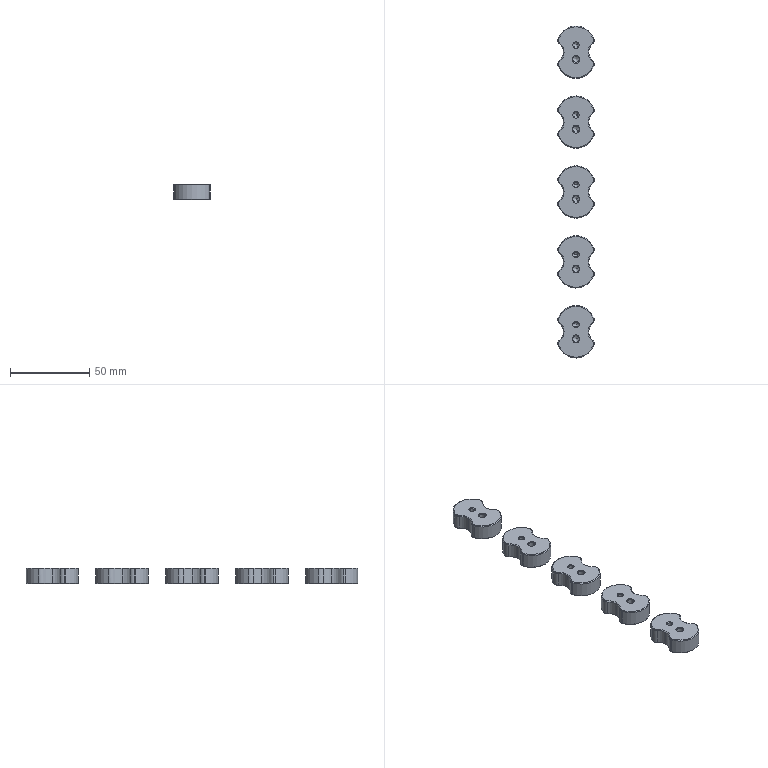NC program | NX | posted with a generic post | part box 22.923 x 209 x 10 mm
Lines 19 to 811 of 9354:
(ZLEVEL_PROFILE_COPY_1 , TOOL : D10)
N36 T15 M6
N38 G54
N40 G17 G0 G90 X-101.822 Y14.358 S9500 M3
N42 G43 Z30. H15
N44 Z1.5
N46 G94 G1 X-101.702 Y14.449 Z1.492 F1000.
N48 X-99.279 Y15.732 Z1.348
N50 X-97.67 Y16.315 Z1.259
N52 X-96.247 Y16.563 Z1.183
N54 X-94.852 Y16.56 Z1.11
N56 X-93.039 Y16.189 Z1.013
N58 X-91.358 Y15.417 Z0.916
N60 X-89.894 Y14.286 Z0.819
N62 X-89.216 Y13.501 Z0.765
N64 X-88.351 Y13.102 Z0.715
N66 X-87.673 Y13.098 Z0.679
N68 X-87.202 Y13.242 Z0.653
N70 X-86.784 Y13.501 Z0.628
N72 X-86.106 Y14.286 Z0.573
N74 X-84.79 Y15.326 Z0.485
N76 X-83.287 Y16.074 Z0.397
N78 X-81.663 Y16.498 Z0.309
N80 X-79.987 Y16.579 Z0.221
N82 X-78.33 Y16.315 Z0.134
N84 X-76.721 Y15.732 Z0.044
N86 X-74.333 Y14.471 Z-0.098
N88 X-72.173 Y12.85 Z-0.239
N90 X-70.294 Y10.91 Z-0.381
N92 X-68.743 Y8.699 Z-0.522
N94 X-67.559 Y6.272 Z-0.664
N96 X-66.772 Y3.688 Z-0.805
N98 X-66.4 Y1.013 Z-0.947
N100 Y0. Z-1.
N102 G2 X-77.674 Y-16.077 R17.1 F3500.
N104 X-86.562 Y-13.758 R8.1
N106 G3 X-89.438 Y-13.758 R1.9
N108 G2 X-98.326 Y-16.077 R8.1
N110 X-98.326 Y16.077 R17.1
N112 X-89.438 Y13.758 R8.1
N114 G3 X-86.562 Y13.758 R1.9
N116 G2 X-77.674 Y16.077 R8.1
N118 X-66.4 Y0. R17.1
N120 G1 X-66.422 Y-0.858 Z-1.007
N122 X-66.486 Y-1.714 Z-1.013
N124 X-66.609 Y-2.666 Z-1.021
N126 X-66.785 Y-3.61 Z-1.028
N128 X-67.014 Y-4.542 Z-1.036
N130 X-67.295 Y-5.46 Z-1.043
N132 X-67.627 Y-6.36 Z-1.05
N134 X-68.009 Y-7.241 Z-1.058
N136 X-68.439 Y-8.098 Z-1.065
N138 X-68.917 Y-8.931 Z-1.073
N140 X-69.441 Y-9.735 Z-1.08
N142 X-70.01 Y-10.508 Z-1.088
N144 X-70.621 Y-11.249 Z-1.095
N146 X-71.272 Y-11.954 Z-1.102
N148 X-71.962 Y-12.621 Z-1.11
N150 X-72.688 Y-13.248 Z-1.117
N152 X-73.449 Y-13.834 Z-1.125
N154 X-74.241 Y-14.376 Z-1.132
N156 X-75.062 Y-14.873 Z-1.14
N158 X-75.91 Y-15.323 Z-1.147
N160 X-76.781 Y-15.725 Z-1.154
N162 X-77.674 Y-16.077 Z-1.162
N164 X-78.255 Y-16.263 Z-1.167
N166 X-78.849 Y-16.405 Z-1.171
N168 X-79.451 Y-16.502 Z-1.176
N170 X-80.06 Y-16.553 Z-1.181
N172 X-80.67 Y-16.558 Z-1.185
N174 X-81.279 Y-16.517 Z-1.19
N176 X-81.883 Y-16.431 Z-1.195
N178 X-82.479 Y-16.299 Z-1.2
N180 X-83.063 Y-16.123 Z-1.204
N182 X-83.632 Y-15.903 Z-1.209
N184 X-84.184 Y-15.641 Z-1.214
N186 X-84.714 Y-15.339 Z-1.219
N188 X-85.219 Y-14.997 Z-1.223
N190 X-85.698 Y-14.618 Z-1.228
N192 X-86.146 Y-14.204 Z-1.233
N194 X-86.562 Y-13.758 Z-1.237
N196 X-86.909 Y-13.444 Z-1.241
N198 X-87.064 Y-13.346 Z-1.242
N200 X-87.429 Y-13.188 Z-1.246
N202 X-87.676 Y-13.128 Z-1.247
N204 X-88.058 Y-13.101 Z-1.25
N206 X-88.324 Y-13.128 Z-1.253
N208 X-88.692 Y-13.23 Z-1.255
N210 X-88.936 Y-13.346 Z-1.258
N212 X-89.08 Y-13.437 Z-1.259
N214 X-89.438 Y-13.758 Z-1.263
N216 X-89.913 Y-14.262 Z-1.268
N218 X-90.43 Y-14.724 Z-1.273
N220 X-90.984 Y-15.141 Z-1.279
N222 X-91.572 Y-15.508 Z-1.284
N224 X-92.189 Y-15.824 Z-1.289
N226 X-92.831 Y-16.086 Z-1.295
N228 X-93.493 Y-16.292 Z-1.3
N230 X-94.17 Y-16.44 Z-1.305
N232 X-94.857 Y-16.53 Z-1.311
N234 X-95.55 Y-16.562 Z-1.316
N236 X-96.021 Y-16.549 Z-1.32
N238 X-96.492 Y-16.509 Z-1.323
N240 X-96.959 Y-16.441 Z-1.327
N242 X-97.421 Y-16.346 Z-1.331
N244 X-97.878 Y-16.225 Z-1.334
N246 X-98.326 Y-16.077 Z-1.338
N248 X-98.977 Y-15.826 Z-1.344
N250 X-99.617 Y-15.549 Z-1.349
N252 X-100.245 Y-15.245 Z-1.354
N254 X-100.861 Y-14.917 Z-1.36
N256 X-101.462 Y-14.563 Z-1.365
N258 X-102.048 Y-14.186 Z-1.371
N260 X-102.854 Y-13.609 Z-1.378
N262 X-103.624 Y-12.987 Z-1.386
N264 X-104.358 Y-12.321 Z-1.394
N266 X-105.051 Y-11.614 Z-1.401
N268 X-105.703 Y-10.867 Z-1.409
N270 X-106.31 Y-10.085 Z-1.417
N272 X-106.87 Y-9.268 Z-1.424
N274 X-107.383 Y-8.421 Z-1.432
N276 X-107.846 Y-7.545 Z-1.44
N278 X-108.257 Y-6.643 Z-1.447
N280 X-108.615 Y-5.72 Z-1.455
N282 X-108.919 Y-4.777 Z-1.463
N284 X-109.168 Y-3.819 Z-1.47
N286 X-109.361 Y-2.847 Z-1.478
N288 X-109.498 Y-1.866 Z-1.486
N290 X-109.577 Y-0.879 Z-1.493
N292 X-109.6 Y0.112 Z-1.501
N294 X-109.564 Y1.101 Z-1.509
N296 X-109.472 Y2.088 Z-1.516
N298 X-109.323 Y3.067 Z-1.524
N300 X-109.117 Y4.036 Z-1.532
N302 X-108.855 Y4.991 Z-1.539
N304 X-108.539 Y5.93 Z-1.547
N306 X-108.169 Y6.849 Z-1.555
N308 X-107.746 Y7.744 Z-1.562
N310 X-107.272 Y8.614 Z-1.57
N312 X-106.748 Y9.455 Z-1.578
N314 X-106.177 Y10.264 Z-1.585
N316 X-105.56 Y11.039 Z-1.593
N318 X-104.899 Y11.776 Z-1.601
N320 X-104.196 Y12.475 Z-1.608
N322 X-103.454 Y13.131 Z-1.616
N324 X-102.675 Y13.743 Z-1.624
N326 X-101.863 Y14.309 Z-1.631
N328 X-101.018 Y14.827 Z-1.639
N330 X-100.146 Y15.296 Z-1.647
N332 X-99.247 Y15.713 Z-1.654
N334 X-98.326 Y16.077 Z-1.662
N336 X-97.878 Y16.225 Z-1.666
N338 X-97.421 Y16.346 Z-1.669
N340 X-96.959 Y16.441 Z-1.673
N342 X-96.492 Y16.509 Z-1.676
N344 X-96.021 Y16.549 Z-1.68
N346 X-95.55 Y16.562 Z-1.684
N348 X-94.857 Y16.53 Z-1.689
N350 X-94.17 Y16.44 Z-1.695
N352 X-93.493 Y16.292 Z-1.7
N354 X-92.831 Y16.086 Z-1.705
N356 X-92.189 Y15.824 Z-1.711
N358 X-91.572 Y15.508 Z-1.716
N360 X-90.984 Y15.141 Z-1.721
N362 X-90.43 Y14.724 Z-1.727
N364 X-89.913 Y14.262 Z-1.732
N366 X-89.438 Y13.758 Z-1.737
N368 X-89.146 Y13.485 Z-1.74
N370 X-89.032 Y13.405 Z-1.742
N372 X-88.74 Y13.25 Z-1.744
N374 X-88.544 Y13.179 Z-1.746
N376 X-88.23 Y13.114 Z-1.748
N378 X-88.012 Y13.1 Z-1.75
N380 X-87.691 Y13.125 Z-1.752
N382 X-87.471 Y13.175 Z-1.754
N384 X-87.172 Y13.29 Z-1.757
N386 X-86.975 Y13.4 Z-1.758
N388 X-86.756 Y13.564 Z-1.76
N390 X-86.562 Y13.758 Z-1.763
N392 X-86.146 Y14.204 Z-1.767
N394 X-85.698 Y14.618 Z-1.772
N396 X-85.219 Y14.997 Z-1.777
N398 X-84.714 Y15.339 Z-1.781
N400 X-84.184 Y15.641 Z-1.786
N402 X-83.632 Y15.903 Z-1.791
N404 X-83.063 Y16.123 Z-1.796
N406 X-82.479 Y16.299 Z-1.8
N408 X-81.883 Y16.431 Z-1.805
N410 X-81.279 Y16.517 Z-1.81
N412 X-80.67 Y16.558 Z-1.815
N414 X-80.06 Y16.553 Z-1.819
N416 X-79.451 Y16.502 Z-1.824
N418 X-78.849 Y16.405 Z-1.829
N420 X-78.255 Y16.263 Z-1.833
N422 X-77.674 Y16.077 Z-1.838
N424 X-76.79 Y15.728 Z-1.845
N426 X-75.926 Y15.331 Z-1.853
N428 X-75.086 Y14.887 Z-1.86
N430 X-74.272 Y14.396 Z-1.868
N432 X-73.486 Y13.861 Z-1.875
N434 X-72.731 Y13.283 Z-1.882
N436 X-72.01 Y12.664 Z-1.89
N438 X-71.324 Y12.006 Z-1.897
N440 X-70.675 Y11.311 Z-1.904
N442 X-70.067 Y10.581 Z-1.912
N444 X-69.499 Y9.818 Z-1.919
N446 X-68.975 Y9.025 Z-1.926
N448 X-68.496 Y8.204 Z-1.934
N450 X-68.064 Y7.357 Z-1.941
N452 X-67.679 Y6.488 Z-1.948
N454 X-67.343 Y5.599 Z-1.956
N456 X-67.056 Y4.693 Z-1.963
N458 X-66.821 Y3.772 Z-1.971
N460 X-66.637 Y2.839 Z-1.978
N462 X-66.506 Y1.898 Z-1.985
N464 X-66.426 Y0.95 Z-1.993
N466 X-66.4 Y0. Z-2.
N468 X-66.422 Y-0.858 Z-2.007
N470 X-66.486 Y-1.714 Z-2.013
N472 X-66.609 Y-2.666 Z-2.021
N474 X-66.785 Y-3.61 Z-2.028
N476 X-67.014 Y-4.542 Z-2.036
N478 X-67.295 Y-5.46 Z-2.043
N480 X-67.627 Y-6.36 Z-2.05
N482 X-68.009 Y-7.241 Z-2.058
N484 X-68.439 Y-8.098 Z-2.065
N486 X-68.917 Y-8.931 Z-2.073
N488 X-69.441 Y-9.735 Z-2.08
N490 X-70.01 Y-10.508 Z-2.088
N492 X-70.621 Y-11.249 Z-2.095
N494 X-71.272 Y-11.954 Z-2.102
N496 X-71.962 Y-12.621 Z-2.11
N498 X-72.688 Y-13.248 Z-2.117
N500 X-73.449 Y-13.834 Z-2.125
N502 X-74.241 Y-14.376 Z-2.132
N504 X-75.062 Y-14.873 Z-2.14
N506 X-75.91 Y-15.323 Z-2.147
N508 X-76.781 Y-15.725 Z-2.154
N510 X-77.674 Y-16.077 Z-2.162
N512 X-78.255 Y-16.263 Z-2.167
N514 X-78.849 Y-16.405 Z-2.171
N516 X-79.451 Y-16.502 Z-2.176
N518 X-80.06 Y-16.553 Z-2.181
N520 X-80.67 Y-16.558 Z-2.185
N522 X-81.279 Y-16.517 Z-2.19
N524 X-81.883 Y-16.431 Z-2.195
N526 X-82.479 Y-16.299 Z-2.2
N528 X-83.063 Y-16.123 Z-2.204
N530 X-83.632 Y-15.903 Z-2.209
N532 X-84.184 Y-15.641 Z-2.214
N534 X-84.714 Y-15.339 Z-2.219
N536 X-85.219 Y-14.997 Z-2.223
N538 X-85.698 Y-14.618 Z-2.228
N540 X-86.146 Y-14.204 Z-2.233
N542 X-86.562 Y-13.758 Z-2.237
N544 X-86.909 Y-13.444 Z-2.241
N546 X-87.064 Y-13.346 Z-2.242
N548 X-87.429 Y-13.188 Z-2.246
N550 X-87.676 Y-13.128 Z-2.247
N552 X-88.058 Y-13.101 Z-2.25
N554 X-88.324 Y-13.128 Z-2.253
N556 X-88.692 Y-13.23 Z-2.255
N558 X-88.936 Y-13.346 Z-2.258
N560 X-89.08 Y-13.437 Z-2.259
N562 X-89.438 Y-13.758 Z-2.263
N564 X-89.913 Y-14.262 Z-2.268
N566 X-90.43 Y-14.724 Z-2.273
N568 X-90.984 Y-15.141 Z-2.279
N570 X-91.572 Y-15.508 Z-2.284
N572 X-92.189 Y-15.824 Z-2.289
N574 X-92.831 Y-16.086 Z-2.295
N576 X-93.493 Y-16.292 Z-2.3
N578 X-94.17 Y-16.44 Z-2.305
N580 X-94.857 Y-16.53 Z-2.311
N582 X-95.55 Y-16.562 Z-2.316
N584 X-96.021 Y-16.549 Z-2.32
N586 X-96.492 Y-16.509 Z-2.323
N588 X-96.959 Y-16.441 Z-2.327
N590 X-97.421 Y-16.346 Z-2.331
N592 X-97.878 Y-16.225 Z-2.334
N594 X-98.326 Y-16.077 Z-2.338
N596 X-98.977 Y-15.826 Z-2.344
N598 X-99.617 Y-15.549 Z-2.349
N600 X-100.245 Y-15.245 Z-2.354
N602 X-100.861 Y-14.917 Z-2.36
N604 X-101.462 Y-14.563 Z-2.365
N606 X-102.048 Y-14.186 Z-2.371
N608 X-102.854 Y-13.609 Z-2.378
N610 X-103.624 Y-12.987 Z-2.386
N612 X-104.358 Y-12.321 Z-2.394
N614 X-105.051 Y-11.614 Z-2.401
N616 X-105.703 Y-10.867 Z-2.409
N618 X-106.31 Y-10.085 Z-2.417
N620 X-106.87 Y-9.268 Z-2.424
N622 X-107.383 Y-8.421 Z-2.432
N624 X-107.846 Y-7.545 Z-2.44
N626 X-108.257 Y-6.643 Z-2.447
N628 X-108.615 Y-5.72 Z-2.455
N630 X-108.919 Y-4.777 Z-2.463
N632 X-109.168 Y-3.819 Z-2.47
N634 X-109.361 Y-2.847 Z-2.478
N636 X-109.498 Y-1.866 Z-2.486
N638 X-109.577 Y-0.879 Z-2.493
N640 X-109.6 Y0.112 Z-2.501
N642 X-109.564 Y1.101 Z-2.509
N644 X-109.472 Y2.088 Z-2.516
N646 X-109.323 Y3.067 Z-2.524
N648 X-109.117 Y4.036 Z-2.532
N650 X-108.855 Y4.991 Z-2.539
N652 X-108.539 Y5.93 Z-2.547
N654 X-108.169 Y6.849 Z-2.555
N656 X-107.746 Y7.744 Z-2.562
N658 X-107.272 Y8.614 Z-2.57
N660 X-106.748 Y9.455 Z-2.578
N662 X-106.177 Y10.264 Z-2.585
N664 X-105.56 Y11.039 Z-2.593
N666 X-104.899 Y11.776 Z-2.601
N668 X-104.196 Y12.475 Z-2.608
N670 X-103.454 Y13.131 Z-2.616
N672 X-102.675 Y13.743 Z-2.624
N674 X-101.863 Y14.309 Z-2.631
N676 X-101.018 Y14.827 Z-2.639
N678 X-100.146 Y15.296 Z-2.647
N680 X-99.247 Y15.713 Z-2.654
N682 X-98.326 Y16.077 Z-2.662
N684 X-97.878 Y16.225 Z-2.666
N686 X-97.421 Y16.346 Z-2.669
N688 X-96.959 Y16.441 Z-2.673
N690 X-96.492 Y16.509 Z-2.676
N692 X-96.021 Y16.549 Z-2.68
N694 X-95.55 Y16.562 Z-2.684
N696 X-94.857 Y16.53 Z-2.689
N698 X-94.17 Y16.44 Z-2.695
N700 X-93.493 Y16.292 Z-2.7
N702 X-92.831 Y16.086 Z-2.705
N704 X-92.189 Y15.824 Z-2.711
N706 X-91.572 Y15.508 Z-2.716
N708 X-90.984 Y15.141 Z-2.721
N710 X-90.43 Y14.724 Z-2.727
N712 X-89.913 Y14.262 Z-2.732
N714 X-89.438 Y13.758 Z-2.737
N716 X-89.146 Y13.485 Z-2.74
N718 X-89.032 Y13.405 Z-2.742
N720 X-88.74 Y13.25 Z-2.744
N722 X-88.544 Y13.179 Z-2.746
N724 X-88.23 Y13.114 Z-2.748
N726 X-88.012 Y13.1 Z-2.75
N728 X-87.691 Y13.125 Z-2.752
N730 X-87.471 Y13.175 Z-2.754
N732 X-87.172 Y13.29 Z-2.757
N734 X-86.975 Y13.4 Z-2.758
N736 X-86.756 Y13.564 Z-2.76
N738 X-86.562 Y13.758 Z-2.763
N740 X-86.146 Y14.204 Z-2.767
N742 X-85.698 Y14.618 Z-2.772
N744 X-85.219 Y14.997 Z-2.777
N746 X-84.714 Y15.339 Z-2.781
N748 X-84.184 Y15.641 Z-2.786
N750 X-83.632 Y15.903 Z-2.791
N752 X-83.063 Y16.123 Z-2.796
N754 X-82.479 Y16.299 Z-2.8
N756 X-81.883 Y16.431 Z-2.805
N758 X-81.279 Y16.517 Z-2.81
N760 X-80.67 Y16.558 Z-2.815
N762 X-80.06 Y16.553 Z-2.819
N764 X-79.451 Y16.502 Z-2.824
N766 X-78.849 Y16.405 Z-2.829
N768 X-78.255 Y16.263 Z-2.833
N770 X-77.674 Y16.077 Z-2.838
N772 X-76.79 Y15.728 Z-2.845
N774 X-75.926 Y15.331 Z-2.853
N776 X-75.086 Y14.887 Z-2.86
N778 X-74.272 Y14.396 Z-2.868
N780 X-73.486 Y13.861 Z-2.875
N782 X-72.731 Y13.283 Z-2.882
N784 X-72.01 Y12.664 Z-2.89
N786 X-71.324 Y12.006 Z-2.897
N788 X-70.675 Y11.311 Z-2.904
N790 X-70.067 Y10.581 Z-2.912
N792 X-69.499 Y9.818 Z-2.919
N794 X-68.975 Y9.025 Z-2.926
N796 X-68.496 Y8.204 Z-2.934
N798 X-68.064 Y7.357 Z-2.941
N800 X-67.679 Y6.488 Z-2.948
N802 X-67.343 Y5.599 Z-2.956
N804 X-67.056 Y4.693 Z-2.963
N806 X-66.821 Y3.772 Z-2.971
N808 X-66.637 Y2.839 Z-2.978
N810 X-66.506 Y1.898 Z-2.985
N812 X-66.426 Y0.95 Z-2.993
N814 X-66.4 Y0. Z-3.
N816 X-66.422 Y-0.858 Z-3.007
N818 X-66.486 Y-1.714 Z-3.013
N820 X-66.609 Y-2.666 Z-3.021
N822 X-66.785 Y-3.61 Z-3.028
N824 X-67.014 Y-4.542 Z-3.036
N826 X-67.295 Y-5.46 Z-3.043
N828 X-67.627 Y-6.36 Z-3.05
N830 X-68.009 Y-7.241 Z-3.058
N832 X-68.439 Y-8.098 Z-3.065
N834 X-68.917 Y-8.931 Z-3.073
N836 X-69.441 Y-9.735 Z-3.08
N838 X-70.01 Y-10.508 Z-3.088
N840 X-70.621 Y-11.249 Z-3.095
N842 X-71.272 Y-11.954 Z-3.102
N844 X-71.962 Y-12.621 Z-3.11
N846 X-72.688 Y-13.248 Z-3.117
N848 X-73.449 Y-13.834 Z-3.125
N850 X-74.241 Y-14.376 Z-3.132
N852 X-75.062 Y-14.873 Z-3.14
N854 X-75.91 Y-15.323 Z-3.147
N856 X-76.781 Y-15.725 Z-3.154
N858 X-77.674 Y-16.077 Z-3.162
N860 X-78.255 Y-16.263 Z-3.167
N862 X-78.849 Y-16.405 Z-3.171
N864 X-79.451 Y-16.502 Z-3.176
N866 X-80.06 Y-16.553 Z-3.181
N868 X-80.67 Y-16.558 Z-3.185
N870 X-81.279 Y-16.517 Z-3.19
N872 X-81.883 Y-16.431 Z-3.195
N874 X-82.479 Y-16.299 Z-3.2
N876 X-83.063 Y-16.123 Z-3.204
N878 X-83.632 Y-15.903 Z-3.209
N880 X-84.184 Y-15.641 Z-3.214
N882 X-84.714 Y-15.339 Z-3.219
N884 X-85.219 Y-14.997 Z-3.223
N886 X-85.698 Y-14.618 Z-3.228
N888 X-86.146 Y-14.204 Z-3.233
N890 X-86.562 Y-13.758 Z-3.237
N892 X-86.909 Y-13.444 Z-3.241
N894 X-87.064 Y-13.346 Z-3.242
N896 X-87.429 Y-13.188 Z-3.246
N898 X-87.676 Y-13.128 Z-3.247
N900 X-88.058 Y-13.101 Z-3.25
N902 X-88.324 Y-13.128 Z-3.253
N904 X-88.692 Y-13.23 Z-3.255
N906 X-88.936 Y-13.346 Z-3.258
N908 X-89.08 Y-13.437 Z-3.259
N910 X-89.438 Y-13.758 Z-3.263
N912 X-89.913 Y-14.262 Z-3.268
N914 X-90.43 Y-14.724 Z-3.273
N916 X-90.984 Y-15.141 Z-3.279
N918 X-91.572 Y-15.508 Z-3.284
N920 X-92.189 Y-15.824 Z-3.289
N922 X-92.831 Y-16.086 Z-3.295
N924 X-93.493 Y-16.292 Z-3.3
N926 X-94.17 Y-16.44 Z-3.305
N928 X-94.857 Y-16.53 Z-3.311
N930 X-95.55 Y-16.562 Z-3.316
N932 X-96.021 Y-16.549 Z-3.32
N934 X-96.492 Y-16.509 Z-3.323
N936 X-96.959 Y-16.441 Z-3.327
N938 X-97.421 Y-16.346 Z-3.331
N940 X-97.878 Y-16.225 Z-3.334
N942 X-98.326 Y-16.077 Z-3.338
N944 X-98.977 Y-15.826 Z-3.344
N946 X-99.617 Y-15.549 Z-3.349
N948 X-100.245 Y-15.245 Z-3.354
N950 X-100.861 Y-14.917 Z-3.36
N952 X-101.462 Y-14.563 Z-3.365
N954 X-102.048 Y-14.186 Z-3.371
N956 X-102.854 Y-13.609 Z-3.378
N958 X-103.624 Y-12.987 Z-3.386
N960 X-104.358 Y-12.321 Z-3.394
N962 X-105.051 Y-11.614 Z-3.401
N964 X-105.703 Y-10.867 Z-3.409
N966 X-106.31 Y-10.085 Z-3.417
N968 X-106.87 Y-9.268 Z-3.424
N970 X-107.383 Y-8.421 Z-3.432
N972 X-107.846 Y-7.545 Z-3.44
N974 X-108.257 Y-6.643 Z-3.447
N976 X-108.615 Y-5.72 Z-3.455
N978 X-108.919 Y-4.777 Z-3.463
N980 X-109.168 Y-3.819 Z-3.47
N982 X-109.361 Y-2.847 Z-3.478
N984 X-109.498 Y-1.866 Z-3.486
N986 X-109.577 Y-0.879 Z-3.493
N988 X-109.6 Y0.112 Z-3.501
N990 X-109.564 Y1.101 Z-3.509
N992 X-109.472 Y2.088 Z-3.516
N994 X-109.323 Y3.067 Z-3.524
N996 X-109.117 Y4.036 Z-3.532
N998 X-108.855 Y4.991 Z-3.539
N1000 X-108.539 Y5.93 Z-3.547
N1002 X-108.169 Y6.849 Z-3.555
N1004 X-107.746 Y7.744 Z-3.562
N1006 X-107.272 Y8.614 Z-3.57
N1008 X-106.748 Y9.455 Z-3.578
N1010 X-106.177 Y10.264 Z-3.585
N1012 X-105.56 Y11.039 Z-3.593
N1014 X-104.899 Y11.776 Z-3.601
N1016 X-104.196 Y12.475 Z-3.608
N1018 X-103.454 Y13.131 Z-3.616
N1020 X-102.675 Y13.743 Z-3.624
N1022 X-101.863 Y14.309 Z-3.631
N1024 X-101.018 Y14.827 Z-3.639
N1026 X-100.146 Y15.296 Z-3.647
N1028 X-99.247 Y15.713 Z-3.654
N1030 X-98.326 Y16.077 Z-3.662
N1032 X-97.878 Y16.225 Z-3.666
N1034 X-97.421 Y16.346 Z-3.669
N1036 X-96.959 Y16.441 Z-3.673
N1038 X-96.492 Y16.509 Z-3.676
N1040 X-96.021 Y16.549 Z-3.68
N1042 X-95.55 Y16.562 Z-3.684
N1044 X-94.857 Y16.53 Z-3.689
N1046 X-94.17 Y16.44 Z-3.695
N1048 X-93.493 Y16.292 Z-3.7
N1050 X-92.831 Y16.086 Z-3.705
N1052 X-92.189 Y15.824 Z-3.711
N1054 X-91.572 Y15.508 Z-3.716
N1056 X-90.984 Y15.141 Z-3.721
N1058 X-90.43 Y14.724 Z-3.727
N1060 X-89.913 Y14.262 Z-3.732
N1062 X-89.438 Y13.758 Z-3.737
N1064 X-89.146 Y13.485 Z-3.74
N1066 X-89.032 Y13.405 Z-3.742
N1068 X-88.74 Y13.25 Z-3.744
N1070 X-88.544 Y13.179 Z-3.746
N1072 X-88.23 Y13.114 Z-3.748
N1074 X-88.012 Y13.1 Z-3.75
N1076 X-87.691 Y13.125 Z-3.752
N1078 X-87.471 Y13.175 Z-3.754
N1080 X-87.172 Y13.29 Z-3.757
N1082 X-86.975 Y13.4 Z-3.758
N1084 X-86.756 Y13.564 Z-3.76
N1086 X-86.562 Y13.758 Z-3.763
N1088 X-86.146 Y14.204 Z-3.767
N1090 X-85.698 Y14.618 Z-3.772
N1092 X-85.219 Y14.997 Z-3.777
N1094 X-84.714 Y15.339 Z-3.781
N1096 X-84.184 Y15.641 Z-3.786
N1098 X-83.632 Y15.903 Z-3.791
N1100 X-83.063 Y16.123 Z-3.796
N1102 X-82.479 Y16.299 Z-3.8
N1104 X-81.883 Y16.431 Z-3.805
N1106 X-81.279 Y16.517 Z-3.81
N1108 X-80.67 Y16.558 Z-3.815
N1110 X-80.06 Y16.553 Z-3.819
N1112 X-79.451 Y16.502 Z-3.824
N1114 X-78.849 Y16.405 Z-3.829
N1116 X-78.255 Y16.263 Z-3.833
N1118 X-77.674 Y16.077 Z-3.838
N1120 X-76.79 Y15.728 Z-3.845
N1122 X-75.926 Y15.331 Z-3.853
N1124 X-75.086 Y14.887 Z-3.86
N1126 X-74.272 Y14.396 Z-3.868
N1128 X-73.486 Y13.861 Z-3.875
N1130 X-72.731 Y13.283 Z-3.882
N1132 X-72.01 Y12.664 Z-3.89
N1134 X-71.324 Y12.006 Z-3.897
N1136 X-70.675 Y11.311 Z-3.904
N1138 X-70.067 Y10.581 Z-3.912
N1140 X-69.499 Y9.818 Z-3.919
N1142 X-68.975 Y9.025 Z-3.926
N1144 X-68.496 Y8.204 Z-3.934
N1146 X-68.064 Y7.357 Z-3.941
N1148 X-67.679 Y6.488 Z-3.948
N1150 X-67.343 Y5.599 Z-3.956
N1152 X-67.056 Y4.693 Z-3.963
N1154 X-66.821 Y3.772 Z-3.971
N1156 X-66.637 Y2.839 Z-3.978
N1158 X-66.506 Y1.898 Z-3.985
N1160 X-66.426 Y0.95 Z-3.993
N1162 X-66.4 Y0. Z-4.
N1164 X-66.422 Y-0.858 Z-4.007
N1166 X-66.486 Y-1.714 Z-4.013
N1168 X-66.609 Y-2.666 Z-4.021
N1170 X-66.785 Y-3.61 Z-4.028
N1172 X-67.014 Y-4.542 Z-4.036
N1174 X-67.295 Y-5.46 Z-4.043
N1176 X-67.627 Y-6.36 Z-4.05
N1178 X-68.009 Y-7.241 Z-4.058
N1180 X-68.439 Y-8.098 Z-4.065
N1182 X-68.917 Y-8.931 Z-4.073
N1184 X-69.441 Y-9.735 Z-4.08
N1186 X-70.01 Y-10.508 Z-4.088
N1188 X-70.621 Y-11.249 Z-4.095
N1190 X-71.272 Y-11.954 Z-4.102
N1192 X-71.962 Y-12.621 Z-4.11
N1194 X-72.688 Y-13.248 Z-4.117
N1196 X-73.449 Y-13.834 Z-4.125
N1198 X-74.241 Y-14.376 Z-4.132
N1200 X-75.062 Y-14.873 Z-4.14
N1202 X-75.91 Y-15.323 Z-4.147
N1204 X-76.781 Y-15.725 Z-4.154
N1206 X-77.674 Y-16.077 Z-4.162
N1208 X-78.255 Y-16.263 Z-4.167
N1210 X-78.849 Y-16.405 Z-4.171
N1212 X-79.451 Y-16.502 Z-4.176
N1214 X-80.06 Y-16.553 Z-4.181
N1216 X-80.67 Y-16.558 Z-4.185
N1218 X-81.279 Y-16.517 Z-4.19
N1220 X-81.883 Y-16.431 Z-4.195
N1222 X-82.479 Y-16.299 Z-4.2
N1224 X-83.063 Y-16.123 Z-4.204
N1226 X-83.632 Y-15.903 Z-4.209
N1228 X-84.184 Y-15.641 Z-4.214
N1230 X-84.714 Y-15.339 Z-4.219
N1232 X-85.219 Y-14.997 Z-4.223
N1234 X-85.698 Y-14.618 Z-4.228
N1236 X-86.146 Y-14.204 Z-4.233
N1238 X-86.562 Y-13.758 Z-4.237
N1240 X-86.909 Y-13.444 Z-4.241
N1242 X-87.064 Y-13.346 Z-4.242
N1244 X-87.429 Y-13.188 Z-4.246
N1246 X-87.676 Y-13.128 Z-4.247
N1248 X-88.058 Y-13.101 Z-4.25
N1250 X-88.324 Y-13.128 Z-4.253
N1252 X-88.692 Y-13.23 Z-4.255
N1254 X-88.936 Y-13.346 Z-4.258
N1256 X-89.08 Y-13.437 Z-4.259
N1258 X-89.438 Y-13.758 Z-4.263
N1260 X-89.913 Y-14.262 Z-4.268
N1262 X-90.43 Y-14.724 Z-4.273
N1264 X-90.984 Y-15.141 Z-4.279
N1266 X-91.572 Y-15.508 Z-4.284
N1268 X-92.189 Y-15.824 Z-4.289
N1270 X-92.831 Y-16.086 Z-4.295
N1272 X-93.493 Y-16.292 Z-4.3
N1274 X-94.17 Y-16.44 Z-4.305
N1276 X-94.857 Y-16.53 Z-4.311
N1278 X-95.55 Y-16.562 Z-4.316
N1280 X-96.021 Y-16.549 Z-4.32
N1282 X-96.492 Y-16.509 Z-4.323
N1284 X-96.959 Y-16.441 Z-4.327
N1286 X-97.421 Y-16.346 Z-4.331
N1288 X-97.878 Y-16.225 Z-4.334
N1290 X-98.326 Y-16.077 Z-4.338
N1292 X-98.977 Y-15.826 Z-4.344
N1294 X-99.617 Y-15.549 Z-4.349
N1296 X-100.245 Y-15.245 Z-4.354
N1298 X-100.861 Y-14.917 Z-4.36
N1300 X-101.462 Y-14.563 Z-4.365
N1302 X-102.048 Y-14.186 Z-4.371
N1304 X-102.854 Y-13.609 Z-4.378
N1306 X-103.624 Y-12.987 Z-4.386
N1308 X-104.358 Y-12.321 Z-4.394
N1310 X-105.051 Y-11.614 Z-4.401
N1312 X-105.703 Y-10.867 Z-4.409
N1314 X-106.31 Y-10.085 Z-4.417
N1316 X-106.87 Y-9.268 Z-4.424
N1318 X-107.383 Y-8.421 Z-4.432
N1320 X-107.846 Y-7.545 Z-4.44
N1322 X-108.257 Y-6.643 Z-4.447
N1324 X-108.615 Y-5.72 Z-4.455
N1326 X-108.919 Y-4.777 Z-4.463
N1328 X-109.168 Y-3.819 Z-4.47
N1330 X-109.361 Y-2.847 Z-4.478
N1332 X-109.498 Y-1.866 Z-4.486
N1334 X-109.577 Y-0.879 Z-4.493
N1336 X-109.6 Y0.112 Z-4.501
N1338 X-109.564 Y1.101 Z-4.509
N1340 X-109.472 Y2.088 Z-4.516
N1342 X-109.323 Y3.067 Z-4.524
N1344 X-109.117 Y4.036 Z-4.532
N1346 X-108.855 Y4.991 Z-4.539
N1348 X-108.539 Y5.93 Z-4.547
N1350 X-108.169 Y6.849 Z-4.555
N1352 X-107.746 Y7.744 Z-4.562
N1354 X-107.272 Y8.614 Z-4.57
N1356 X-106.748 Y9.455 Z-4.578
N1358 X-106.177 Y10.264 Z-4.585
N1360 X-105.56 Y11.039 Z-4.593
N1362 X-104.899 Y11.776 Z-4.601
N1364 X-104.196 Y12.475 Z-4.608
N1366 X-103.454 Y13.131 Z-4.616
N1368 X-102.675 Y13.743 Z-4.624
N1370 X-101.863 Y14.309 Z-4.631
N1372 X-101.018 Y14.827 Z-4.639
N1374 X-100.146 Y15.296 Z-4.647
N1376 X-99.247 Y15.713 Z-4.654
N1378 X-98.326 Y16.077 Z-4.662
N1380 X-97.878 Y16.225 Z-4.666
N1382 X-97.421 Y16.346 Z-4.669
N1384 X-96.959 Y16.441 Z-4.673
N1386 X-96.492 Y16.509 Z-4.676
N1388 X-96.021 Y16.549 Z-4.68
N1390 X-95.55 Y16.562 Z-4.684
N1392 X-94.857 Y16.53 Z-4.689
N1394 X-94.17 Y16.44 Z-4.695
N1396 X-93.493 Y16.292 Z-4.7
N1398 X-92.831 Y16.086 Z-4.705
N1400 X-92.189 Y15.824 Z-4.711
N1402 X-91.572 Y15.508 Z-4.716
N1404 X-90.984 Y15.141 Z-4.721
N1406 X-90.43 Y14.724 Z-4.727
N1408 X-89.913 Y14.262 Z-4.732
N1410 X-89.438 Y13.758 Z-4.737
N1412 X-89.146 Y13.485 Z-4.74
N1414 X-89.032 Y13.405 Z-4.742
N1416 X-88.74 Y13.25 Z-4.744
N1418 X-88.544 Y13.179 Z-4.746
N1420 X-88.23 Y13.114 Z-4.748
N1422 X-88.012 Y13.1 Z-4.75
N1424 X-87.691 Y13.125 Z-4.752
N1426 X-87.471 Y13.175 Z-4.754
N1428 X-87.172 Y13.29 Z-4.757
N1430 X-86.975 Y13.4 Z-4.758
N1432 X-86.756 Y13.564 Z-4.76
N1434 X-86.562 Y13.758 Z-4.763
N1436 X-86.146 Y14.204 Z-4.767
N1438 X-85.698 Y14.618 Z-4.772
N1440 X-85.219 Y14.997 Z-4.777
N1442 X-84.714 Y15.339 Z-4.781
N1444 X-84.184 Y15.641 Z-4.786
N1446 X-83.632 Y15.903 Z-4.791
N1448 X-83.063 Y16.123 Z-4.796
N1450 X-82.479 Y16.299 Z-4.8
N1452 X-81.883 Y16.431 Z-4.805
N1454 X-81.279 Y16.517 Z-4.81
N1456 X-80.67 Y16.558 Z-4.815
N1458 X-80.06 Y16.553 Z-4.819
N1460 X-79.451 Y16.502 Z-4.824
N1462 X-78.849 Y16.405 Z-4.829
N1464 X-78.255 Y16.263 Z-4.833
N1466 X-77.674 Y16.077 Z-4.838
N1468 X-76.79 Y15.728 Z-4.845
N1470 X-75.926 Y15.331 Z-4.853
N1472 X-75.086 Y14.887 Z-4.86
N1474 X-74.272 Y14.396 Z-4.868
N1476 X-73.486 Y13.861 Z-4.875
N1478 X-72.731 Y13.283 Z-4.882
N1480 X-72.01 Y12.664 Z-4.89
N1482 X-71.324 Y12.006 Z-4.897
N1484 X-70.675 Y11.311 Z-4.904
N1486 X-70.067 Y10.581 Z-4.912
N1488 X-69.499 Y9.818 Z-4.919
N1490 X-68.975 Y9.025 Z-4.926
N1492 X-68.496 Y8.204 Z-4.934
N1494 X-68.064 Y7.357 Z-4.941
N1496 X-67.679 Y6.488 Z-4.948
N1498 X-67.343 Y5.599 Z-4.956
N1500 X-67.056 Y4.693 Z-4.963
N1502 X-66.821 Y3.772 Z-4.971
N1504 X-66.637 Y2.839 Z-4.978
N1506 X-66.506 Y1.898 Z-4.985
N1508 X-66.426 Y0.95 Z-4.993
N1510 X-66.4 Y0. Z-5.
N1512 X-66.422 Y-0.858 Z-5.007
N1514 X-66.486 Y-1.714 Z-5.013
N1516 X-66.609 Y-2.666 Z-5.021
N1518 X-66.785 Y-3.61 Z-5.028
N1520 X-67.014 Y-4.542 Z-5.036
N1522 X-67.295 Y-5.46 Z-5.043
N1524 X-67.627 Y-6.36 Z-5.05
N1526 X-68.009 Y-7.241 Z-5.058
N1528 X-68.439 Y-8.098 Z-5.065
N1530 X-68.917 Y-8.931 Z-5.073
N1532 X-69.441 Y-9.735 Z-5.08
N1534 X-70.01 Y-10.508 Z-5.088
N1536 X-70.621 Y-11.249 Z-5.095
N1538 X-71.272 Y-11.954 Z-5.102
N1540 X-71.962 Y-12.621 Z-5.11
N1542 X-72.688 Y-13.248 Z-5.117
N1544 X-73.449 Y-13.834 Z-5.125
N1546 X-74.241 Y-14.376 Z-5.132
N1548 X-75.062 Y-14.873 Z-5.14
N1550 X-75.91 Y-15.323 Z-5.147
N1552 X-76.781 Y-15.725 Z-5.154
N1554 X-77.674 Y-16.077 Z-5.162
N1556 X-78.255 Y-16.263 Z-5.167
N1558 X-78.849 Y-16.405 Z-5.171
N1560 X-79.451 Y-16.502 Z-5.176
N1562 X-80.06 Y-16.553 Z-5.181
N1564 X-80.67 Y-16.558 Z-5.185
N1566 X-81.279 Y-16.517 Z-5.19
N1568 X-81.883 Y-16.431 Z-5.195
N1570 X-82.479 Y-16.299 Z-5.2
N1572 X-83.063 Y-16.123 Z-5.204
N1574 X-83.632 Y-15.903 Z-5.209
N1576 X-84.184 Y-15.641 Z-5.214
N1578 X-84.714 Y-15.339 Z-5.219
N1580 X-85.219 Y-14.997 Z-5.223
N1582 X-85.698 Y-14.618 Z-5.228
N1584 X-86.146 Y-14.204 Z-5.233
N1586 X-86.562 Y-13.758 Z-5.237
N1588 X-86.909 Y-13.444 Z-5.241
N1590 X-87.064 Y-13.346 Z-5.242
N1592 X-87.429 Y-13.188 Z-5.246
N1594 X-87.676 Y-13.128 Z-5.247
N1596 X-88.058 Y-13.101 Z-5.25
N1598 X-88.324 Y-13.128 Z-5.253
N1600 X-88.692 Y-13.23 Z-5.255
N1602 X-88.936 Y-13.346 Z-5.258
N1604 X-89.08 Y-13.437 Z-5.259
N1606 X-89.438 Y-13.758 Z-5.263
N1608 X-89.913 Y-14.262 Z-5.268
N1610 X-90.43 Y-14.724 Z-5.273
N1612 X-90.984 Y-15.141 Z-5.279
N1614 X-91.572 Y-15.508 Z-5.284